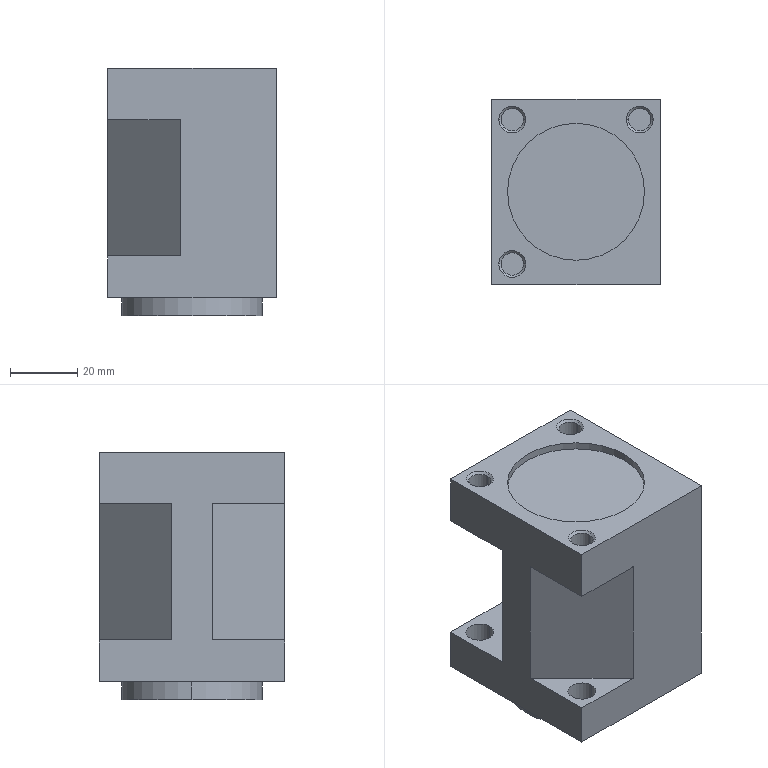Part | STEP file | GRM4_B10_BODYOPTION_M | 1 solid | 57 faces | box 50.292 x 55.27 x 73.66 mm | volume 161375 mm3 | plane 23 | cylinder 22 | cone 12 | commonest cylinder face diameters 6.647 x6 8.331 x6 8.566 x6 40.767 x2 41.885 x2